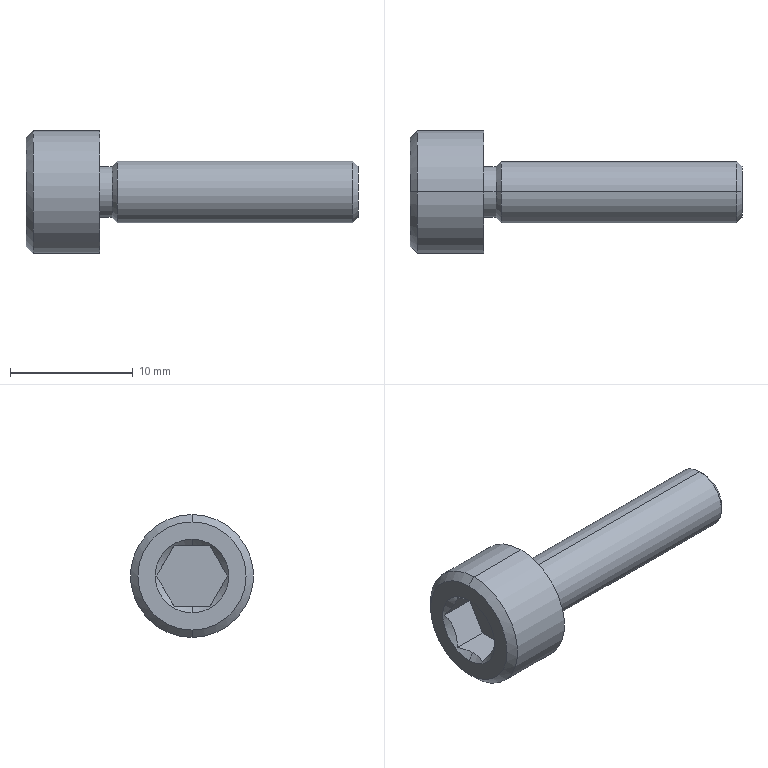Part | STEP file | LFSP35B20boltbolt | 1 solid | 24 faces | box 27 x 10 x 10 mm | volume 802.883 mm3 | plane 10 | cone 8 | cylinder 6 | commonest cylinder face diameters 4.134 x2 5 x2 10 x2